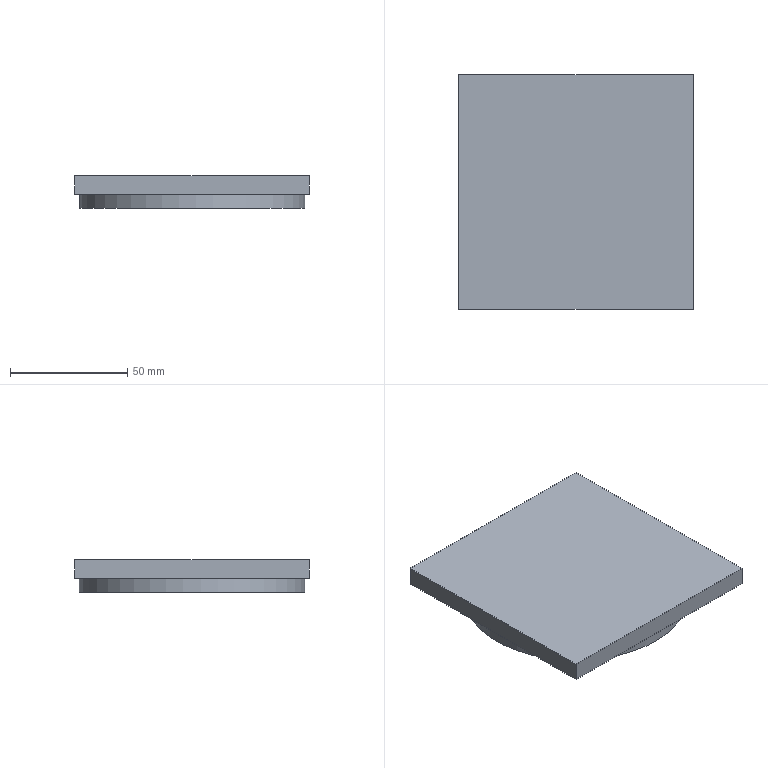Part | NX | 2 solids | 27 faces | box 100 x 100 x 14 mm | volume 81891 mm3 | cylinder 15 | plane 12 | commonest cylinder face diameters 4.3 x6 5.5 x3 11 x3 96 x2 48.3 x1
STEP:
#1=CARTESIAN_POINT('',(48.,0.,4.));
#2=VERTEX_POINT('',#1);
#3=CARTESIAN_POINT('',(0.,0.,4.));
#4=DIRECTION('',(0.,0.,1.));
#5=DIRECTION('',(1.,0.,0.));
#6=AXIS2_PLACEMENT_3D('',#3,#4,#5);
#7=CIRCLE('',#6,48.);
#8=EDGE_CURVE('',#2,#2,#7,.F.);
#9=ORIENTED_EDGE('',*,*,#8,.F.);
#10=EDGE_LOOP('',(#9));
#11=FACE_BOUND('',#10,.T.);
#12=CARTESIAN_POINT('',(48.,0.,0.));
#13=VERTEX_POINT('',#12);
#14=CARTESIAN_POINT('',(0.,0.,0.));
#15=DIRECTION('',(0.,0.,1.));
#16=DIRECTION('',(1.,0.,0.));
#17=AXIS2_PLACEMENT_3D('',#14,#15,#16);
#18=CIRCLE('',#17,48.);
#19=EDGE_CURVE('',#13,#13,#18,.T.);
#20=ORIENTED_EDGE('',*,*,#19,.F.);
#21=EDGE_LOOP('',(#20));
#22=FACE_BOUND('',#21,.T.);
#23=CARTESIAN_POINT('',(0.,0.,4.));
#24=DIRECTION('',(0.,0.,-1.));
#25=DIRECTION('',(-1.,0.,0.));
#26=AXIS2_PLACEMENT_3D('',#23,#24,#25);
#27=CYLINDRICAL_SURFACE('',#26,48.);
#28=ADVANCED_FACE('',(#11,#22),#27,.F.);
#29=ORIENTED_EDGE('',*,*,#8,.T.);
#30=EDGE_LOOP('',(#29));
#31=FACE_BOUND('',#30,.T.);
#32=CARTESIAN_POINT('',(0.,0.,4.));
#33=DIRECTION('',(0.,0.,1.));
#34=DIRECTION('',(1.,0.,0.));
#35=AXIS2_PLACEMENT_3D('',#32,#33,#34);
#36=PLANE('',#35);
#37=ADVANCED_FACE('',(#31),#36,.F.);
#38=CARTESIAN_POINT('',(50.,-50.,8.));
#39=VERTEX_POINT('',#38);
#40=CARTESIAN_POINT('',(50.,50.,8.));
#41=VERTEX_POINT('',#40);
#42=CARTESIAN_POINT('',(50.,-50.,8.));
#43=DIRECTION('',(0.,1.,0.));
#44=VECTOR('',#43,1000.);
#45=LINE('',#42,#44);
#46=EDGE_CURVE('',#39,#41,#45,.T.);
#47=ORIENTED_EDGE('',*,*,#46,.T.);
#48=CARTESIAN_POINT('',(-50.,50.,8.));
#49=VERTEX_POINT('',#48);
#50=CARTESIAN_POINT('',(50.,50.,8.));
#51=DIRECTION('',(-1.,0.,0.));
#52=VECTOR('',#51,1000.);
#53=LINE('',#50,#52);
#54=EDGE_CURVE('',#41,#49,#53,.T.);
#55=ORIENTED_EDGE('',*,*,#54,.T.);
#56=CARTESIAN_POINT('',(-50.,-50.,8.));
#57=VERTEX_POINT('',#56);
#58=CARTESIAN_POINT('',(-50.,50.,8.));
#59=DIRECTION('',(0.,-1.,0.));
#60=VECTOR('',#59,1000.);
#61=LINE('',#58,#60);
#62=EDGE_CURVE('',#49,#57,#61,.T.);
#63=ORIENTED_EDGE('',*,*,#62,.T.);
#64=CARTESIAN_POINT('',(-50.,-50.,8.));
#65=DIRECTION('',(1.,0.,0.));
#66=VECTOR('',#65,1000.);
#67=LINE('',#64,#66);
#68=EDGE_CURVE('',#57,#39,#67,.T.);
#69=ORIENTED_EDGE('',*,*,#68,.T.);
#70=EDGE_LOOP('',(#47,#55,#63,#69));
#71=FACE_BOUND('',#70,.T.);
#72=CARTESIAN_POINT('',(0.,0.,8.));
#73=DIRECTION('',(0.,0.,1.));
#74=DIRECTION('',(1.,0.,0.));
#75=AXIS2_PLACEMENT_3D('',#72,#73,#74);
#76=PLANE('',#75);
#77=ADVANCED_FACE('',(#71),#76,.T.);
#78=CARTESIAN_POINT('',(50.,50.,0.));
#79=VERTEX_POINT('',#78);
#80=CARTESIAN_POINT('',(-50.,50.,0.));
#81=VERTEX_POINT('',#80);
#82=CARTESIAN_POINT('',(50.,50.,0.));
#83=DIRECTION('',(-1.,0.,0.));
#84=VECTOR('',#83,1000.);
#85=LINE('',#82,#84);
#86=EDGE_CURVE('',#79,#81,#85,.T.);
#87=ORIENTED_EDGE('',*,*,#86,.T.);
#88=CARTESIAN_POINT('',(-50.,50.,8.));
#89=DIRECTION('',(0.,0.,-1.));
#90=VECTOR('',#89,1000.);
#91=LINE('',#88,#90);
#92=EDGE_CURVE('',#49,#81,#91,.T.);
#93=ORIENTED_EDGE('',*,*,#92,.F.);
#94=ORIENTED_EDGE('',*,*,#54,.F.);
#95=CARTESIAN_POINT('',(50.,50.,8.));
#96=DIRECTION('',(0.,0.,-1.));
#97=VECTOR('',#96,1000.);
#98=LINE('',#95,#97);
#99=EDGE_CURVE('',#41,#79,#98,.T.);
#100=ORIENTED_EDGE('',*,*,#99,.T.);
#101=EDGE_LOOP('',(#87,#93,#94,#100));
#102=FACE_BOUND('',#101,.T.);
#103=CARTESIAN_POINT('',(50.,50.,8.));
#104=DIRECTION('',(0.,-1.,0.));
#105=DIRECTION('',(0.,0.,-1.));
#106=AXIS2_PLACEMENT_3D('',#103,#104,#105);
#107=PLANE('',#106);
#108=ADVANCED_FACE('',(#102),#107,.F.);
#109=CARTESIAN_POINT('',(-50.,-50.,0.));
#110=VERTEX_POINT('',#109);
#111=CARTESIAN_POINT('',(-50.,50.,0.));
#112=DIRECTION('',(0.,-1.,0.));
#113=VECTOR('',#112,1000.);
#114=LINE('',#111,#113);
#115=EDGE_CURVE('',#81,#110,#114,.T.);
#116=ORIENTED_EDGE('',*,*,#115,.T.);
#117=CARTESIAN_POINT('',(-50.,-50.,8.));
#118=DIRECTION('',(0.,0.,-1.));
#119=VECTOR('',#118,1000.);
#120=LINE('',#117,#119);
#121=EDGE_CURVE('',#57,#110,#120,.T.);
#122=ORIENTED_EDGE('',*,*,#121,.F.);
#123=ORIENTED_EDGE('',*,*,#62,.F.);
#124=ORIENTED_EDGE('',*,*,#92,.T.);
#125=EDGE_LOOP('',(#116,#122,#123,#124));
#126=FACE_BOUND('',#125,.T.);
#127=CARTESIAN_POINT('',(-50.,50.,8.));
#128=DIRECTION('',(1.,0.,0.));
#129=DIRECTION('',(0.,0.,-1.));
#130=AXIS2_PLACEMENT_3D('',#127,#128,#129);
#131=PLANE('',#130);
#132=ADVANCED_FACE('',(#126),#131,.F.);
#133=CARTESIAN_POINT('',(50.,-50.,0.));
#134=VERTEX_POINT('',#133);
#135=CARTESIAN_POINT('',(-50.,-50.,0.));
#136=DIRECTION('',(1.,0.,0.));
#137=VECTOR('',#136,1000.);
#138=LINE('',#135,#137);
#139=EDGE_CURVE('',#110,#134,#138,.T.);
#140=ORIENTED_EDGE('',*,*,#139,.T.);
#141=CARTESIAN_POINT('',(50.,-50.,8.));
#142=DIRECTION('',(0.,0.,-1.));
#143=VECTOR('',#142,1000.);
#144=LINE('',#141,#143);
#145=EDGE_CURVE('',#39,#134,#144,.T.);
#146=ORIENTED_EDGE('',*,*,#145,.F.);
#147=ORIENTED_EDGE('',*,*,#68,.F.);
#148=ORIENTED_EDGE('',*,*,#121,.T.);
#149=EDGE_LOOP('',(#140,#146,#147,#148));
#150=FACE_BOUND('',#149,.T.);
#151=CARTESIAN_POINT('',(-50.,-50.,8.));
#152=DIRECTION('',(0.,1.,0.));
#153=DIRECTION('',(0.,0.,1.));
#154=AXIS2_PLACEMENT_3D('',#151,#152,#153);
#155=PLANE('',#154);
#156=ADVANCED_FACE('',(#150),#155,.F.);
#157=CARTESIAN_POINT('',(50.,-50.,0.));
#158=DIRECTION('',(0.,1.,0.));
#159=VECTOR('',#158,1000.);
#160=LINE('',#157,#159);
#161=EDGE_CURVE('',#134,#79,#160,.T.);
#162=ORIENTED_EDGE('',*,*,#161,.T.);
#163=ORIENTED_EDGE('',*,*,#99,.F.);
#164=ORIENTED_EDGE('',*,*,#46,.F.);
#165=ORIENTED_EDGE('',*,*,#145,.T.);
#166=EDGE_LOOP('',(#162,#163,#164,#165));
#167=FACE_BOUND('',#166,.T.);
#168=CARTESIAN_POINT('',(50.,-50.,8.));
#169=DIRECTION('',(-1.,0.,0.));
#170=DIRECTION('',(0.,0.,1.));
#171=AXIS2_PLACEMENT_3D('',#168,#169,#170);
#172=PLANE('',#171);
#173=ADVANCED_FACE('',(#167),#172,.F.);
#174=ORIENTED_EDGE('',*,*,#19,.T.);
#175=EDGE_LOOP('',(#174));
#176=FACE_BOUND('',#175,.T.);
#177=ORIENTED_EDGE('',*,*,#161,.F.);
#178=ORIENTED_EDGE('',*,*,#139,.F.);
#179=ORIENTED_EDGE('',*,*,#115,.F.);
#180=ORIENTED_EDGE('',*,*,#86,.F.);
#181=EDGE_LOOP('',(#177,#178,#179,#180));
#182=FACE_BOUND('',#181,.T.);
#183=CARTESIAN_POINT('',(0.,0.,0.));
#184=DIRECTION('',(0.,0.,1.));
#185=DIRECTION('',(1.,0.,0.));
#186=AXIS2_PLACEMENT_3D('',#183,#184,#185);
#187=PLANE('',#186);
#188=ADVANCED_FACE('',(#176,#182),#187,.F.);
#189=CLOSED_SHELL('',(#28,#37,#77,#108,#132,#156,#173,#188));
#190=MANIFOLD_SOLID_BREP('',#189);
#191=CARTESIAN_POINT('',(-22.225,-38.495,-6.));
#192=VERTEX_POINT('',#191);
#193=CARTESIAN_POINT('',(-20.85,-36.113,-6.));
#194=DIRECTION('',(0.,0.,1.));
#195=DIRECTION('',(-0.5,-0.866,0.));
#196=AXIS2_PLACEMENT_3D('',#193,#194,#195);
#197=CIRCLE('',#196,2.75);
#198=EDGE_CURVE('',#192,#192,#197,.T.);
#199=ORIENTED_EDGE('',*,*,#198,.F.);
#200=EDGE_LOOP('',(#199));
#201=FACE_BOUND('',#200,.T.);
#202=CARTESIAN_POINT('',(-18.1,-36.113,-3.));
#203=VERTEX_POINT('',#202);
#204=CARTESIAN_POINT('',(-20.85,-36.113,-3.));
#205=DIRECTION('',(0.,0.,1.));
#206=DIRECTION('',(1.,0.,0.));
#207=AXIS2_PLACEMENT_3D('',#204,#205,#206);
#208=CIRCLE('',#207,2.75);
#209=EDGE_CURVE('',#203,#203,#208,.F.);
#210=ORIENTED_EDGE('',*,*,#209,.F.);
#211=EDGE_LOOP('',(#210));
#212=FACE_BOUND('',#211,.T.);
#213=CARTESIAN_POINT('',(-20.85,-36.113,-6.));
#214=DIRECTION('',(0.,0.,1.));
#215=DIRECTION('',(1.,0.,0.));
#216=AXIS2_PLACEMENT_3D('',#213,#214,#215);
#217=CYLINDRICAL_SURFACE('',#216,2.75);
#218=ADVANCED_FACE('',(#201,#212),#217,.F.);
#219=CARTESIAN_POINT('',(44.45,0.,-6.));
#220=VERTEX_POINT('',#219);
#221=CARTESIAN_POINT('',(41.7,0.,-6.));
#222=DIRECTION('',(0.,0.,1.));
#223=DIRECTION('',(1.,0.,0.));
#224=AXIS2_PLACEMENT_3D('',#221,#222,#223);
#225=CIRCLE('',#224,2.75);
#226=EDGE_CURVE('',#220,#220,#225,.T.);
#227=ORIENTED_EDGE('',*,*,#226,.F.);
#228=EDGE_LOOP('',(#227));
#229=FACE_BOUND('',#228,.T.);
#230=CARTESIAN_POINT('',(44.45,0.,-3.));
#231=VERTEX_POINT('',#230);
#232=CARTESIAN_POINT('',(41.7,0.,-3.));
#233=DIRECTION('',(0.,0.,1.));
#234=DIRECTION('',(1.,0.,0.));
#235=AXIS2_PLACEMENT_3D('',#232,#233,#234);
#236=CIRCLE('',#235,2.75);
#237=EDGE_CURVE('',#231,#231,#236,.F.);
#238=ORIENTED_EDGE('',*,*,#237,.F.);
#239=EDGE_LOOP('',(#238));
#240=FACE_BOUND('',#239,.T.);
#241=CARTESIAN_POINT('',(41.7,0.,-6.));
#242=DIRECTION('',(0.,0.,1.));
#243=DIRECTION('',(1.,0.,0.));
#244=AXIS2_PLACEMENT_3D('',#241,#242,#243);
#245=CYLINDRICAL_SURFACE('',#244,2.75);
#246=ADVANCED_FACE('',(#229,#240),#245,.F.);
#247=CARTESIAN_POINT('',(-23.174,15.862,-6.));
#248=VERTEX_POINT('',#247);
#249=CARTESIAN_POINT('',(-24.249,14.,-6.));
#250=DIRECTION('',(0.,0.,1.));
#251=DIRECTION('',(0.5,0.866,0.));
#252=AXIS2_PLACEMENT_3D('',#249,#250,#251);
#253=CIRCLE('',#252,2.15);
#254=EDGE_CURVE('',#248,#248,#253,.T.);
#255=ORIENTED_EDGE('',*,*,#254,.F.);
#256=EDGE_LOOP('',(#255));
#257=FACE_BOUND('',#256,.T.);
#258=CARTESIAN_POINT('',(-23.174,15.862,0.));
#259=VERTEX_POINT('',#258);
#260=CARTESIAN_POINT('',(-24.249,14.,0.));
#261=DIRECTION('',(0.,0.,1.));
#262=DIRECTION('',(0.5,0.866,0.));
#263=AXIS2_PLACEMENT_3D('',#260,#261,#262);
#264=CIRCLE('',#263,2.15);
#265=EDGE_CURVE('',#259,#259,#264,.T.);
#266=ORIENTED_EDGE('',*,*,#265,.T.);
#267=EDGE_LOOP('',(#266));
#268=FACE_BOUND('',#267,.T.);
#269=CARTESIAN_POINT('',(-24.249,14.,-6.));
#270=DIRECTION('',(0.,0.,1.));
#271=DIRECTION('',(1.,0.,0.));
#272=AXIS2_PLACEMENT_3D('',#269,#270,#271);
#273=CYLINDRICAL_SURFACE('',#272,2.15);
#274=ADVANCED_FACE('',(#257,#268),#273,.F.);
#275=CARTESIAN_POINT('',(24.15,0.,-6.));
#276=VERTEX_POINT('',#275);
#277=CARTESIAN_POINT('',(0.,0.,-6.));
#278=DIRECTION('',(0.,0.,1.));
#279=DIRECTION('',(1.,0.,0.));
#280=AXIS2_PLACEMENT_3D('',#277,#278,#279);
#281=CIRCLE('',#280,24.15);
#282=EDGE_CURVE('',#276,#276,#281,.T.);
#283=ORIENTED_EDGE('',*,*,#282,.F.);
#284=EDGE_LOOP('',(#283));
#285=FACE_BOUND('',#284,.T.);
#286=CARTESIAN_POINT('',(24.15,0.,0.));
#287=VERTEX_POINT('',#286);
#288=CARTESIAN_POINT('',(0.,0.,0.));
#289=DIRECTION('',(0.,0.,1.));
#290=DIRECTION('',(1.,0.,0.));
#291=AXIS2_PLACEMENT_3D('',#288,#289,#290);
#292=CIRCLE('',#291,24.15);
#293=EDGE_CURVE('',#287,#287,#292,.T.);
#294=ORIENTED_EDGE('',*,*,#293,.T.);
#295=EDGE_LOOP('',(#294));
#296=FACE_BOUND('',#295,.T.);
#297=CARTESIAN_POINT('',(0.,0.,-6.));
#298=DIRECTION('',(0.,0.,1.));
#299=DIRECTION('',(1.,0.,0.));
#300=AXIS2_PLACEMENT_3D('',#297,#298,#299);
#301=CYLINDRICAL_SURFACE('',#300,24.15);
#302=ADVANCED_FACE('',(#285,#296),#301,.F.);
#303=CARTESIAN_POINT('',(-23.6,36.113,-3.));
#304=VERTEX_POINT('',#303);
#305=CARTESIAN_POINT('',(-20.85,36.113,-3.));
#306=DIRECTION('',(0.,0.,-1.));
#307=DIRECTION('',(-1.,0.,0.));
#308=AXIS2_PLACEMENT_3D('',#305,#306,#307);
#309=CIRCLE('',#308,2.75);
#310=EDGE_CURVE('',#304,#304,#309,.F.);
#311=ORIENTED_EDGE('',*,*,#310,.T.);
#312=EDGE_LOOP('',(#311));
#313=FACE_BOUND('',#312,.T.);
#314=CARTESIAN_POINT('',(-22.225,38.495,-6.));
#315=VERTEX_POINT('',#314);
#316=CARTESIAN_POINT('',(-20.85,36.113,-6.));
#317=DIRECTION('',(0.,0.,1.));
#318=DIRECTION('',(-0.5,0.866,0.));
#319=AXIS2_PLACEMENT_3D('',#316,#317,#318);
#320=CIRCLE('',#319,2.75);
#321=EDGE_CURVE('',#315,#315,#320,.T.);
#322=ORIENTED_EDGE('',*,*,#321,.F.);
#323=EDGE_LOOP('',(#322));
#324=FACE_BOUND('',#323,.T.);
#325=CARTESIAN_POINT('',(-20.85,36.113,-6.));
#326=DIRECTION('',(0.,0.,1.));
#327=DIRECTION('',(1.,0.,0.));
#328=AXIS2_PLACEMENT_3D('',#325,#326,#327);
#329=CYLINDRICAL_SURFACE('',#328,2.75);
#330=ADVANCED_FACE('',(#313,#324),#329,.F.);
#331=CARTESIAN_POINT('',(-2.15,-28.,-6.));
#332=VERTEX_POINT('',#331);
#333=CARTESIAN_POINT('',(0.,-28.,-6.));
#334=DIRECTION('',(0.,0.,1.));
#335=DIRECTION('',(-1.,0.,0.));
#336=AXIS2_PLACEMENT_3D('',#333,#334,#335);
#337=CIRCLE('',#336,2.15);
#338=EDGE_CURVE('',#332,#332,#337,.T.);
#339=ORIENTED_EDGE('',*,*,#338,.F.);
#340=EDGE_LOOP('',(#339));
#341=FACE_BOUND('',#340,.T.);
#342=CARTESIAN_POINT('',(-2.15,-28.,0.));
#343=VERTEX_POINT('',#342);
#344=CARTESIAN_POINT('',(0.,-28.,0.));
#345=DIRECTION('',(0.,0.,1.));
#346=DIRECTION('',(-1.,0.,0.));
#347=AXIS2_PLACEMENT_3D('',#344,#345,#346);
#348=CIRCLE('',#347,2.15);
#349=EDGE_CURVE('',#343,#343,#348,.T.);
#350=ORIENTED_EDGE('',*,*,#349,.T.);
#351=EDGE_LOOP('',(#350));
#352=FACE_BOUND('',#351,.T.);
#353=CARTESIAN_POINT('',(0.,-28.,-6.));
#354=DIRECTION('',(0.,0.,1.));
#355=DIRECTION('',(1.,0.,0.));
#356=AXIS2_PLACEMENT_3D('',#353,#354,#355);
#357=CYLINDRICAL_SURFACE('',#356,2.15);
#358=ADVANCED_FACE('',(#341,#352),#357,.F.);
#359=CARTESIAN_POINT('',(2.15,28.,-6.));
#360=VERTEX_POINT('',#359);
#361=CARTESIAN_POINT('',(0.,28.,-6.));
#362=DIRECTION('',(0.,0.,1.));
#363=DIRECTION('',(1.,0.,0.));
#364=AXIS2_PLACEMENT_3D('',#361,#362,#363);
#365=CIRCLE('',#364,2.15);
#366=EDGE_CURVE('',#360,#360,#365,.T.);
#367=ORIENTED_EDGE('',*,*,#366,.F.);
#368=EDGE_LOOP('',(#367));
#369=FACE_BOUND('',#368,.T.);
#370=CARTESIAN_POINT('',(2.15,28.,0.));
#371=VERTEX_POINT('',#370);
#372=CARTESIAN_POINT('',(0.,28.,0.));
#373=DIRECTION('',(0.,0.,1.));
#374=DIRECTION('',(1.,0.,0.));
#375=AXIS2_PLACEMENT_3D('',#372,#373,#374);
#376=CIRCLE('',#375,2.15);
#377=EDGE_CURVE('',#371,#371,#376,.T.);
#378=ORIENTED_EDGE('',*,*,#377,.T.);
#379=EDGE_LOOP('',(#378));
#380=FACE_BOUND('',#379,.T.);
#381=CARTESIAN_POINT('',(0.,28.,-6.));
#382=DIRECTION('',(0.,0.,1.));
#383=DIRECTION('',(1.,0.,0.));
#384=AXIS2_PLACEMENT_3D('',#381,#382,#383);
#385=CYLINDRICAL_SURFACE('',#384,2.15);
#386=ADVANCED_FACE('',(#369,#380),#385,.F.);
#387=CARTESIAN_POINT('',(23.174,-15.862,-6.));
#388=VERTEX_POINT('',#387);
#389=CARTESIAN_POINT('',(24.249,-14.,-6.));
#390=DIRECTION('',(0.,0.,1.));
#391=DIRECTION('',(-0.5,-0.866,0.));
#392=AXIS2_PLACEMENT_3D('',#389,#390,#391);
#393=CIRCLE('',#392,2.15);
#394=EDGE_CURVE('',#388,#388,#393,.T.);
#395=ORIENTED_EDGE('',*,*,#394,.F.);
#396=EDGE_LOOP('',(#395));
#397=FACE_BOUND('',#396,.T.);
#398=CARTESIAN_POINT('',(23.174,-15.862,0.));
#399=VERTEX_POINT('',#398);
#400=CARTESIAN_POINT('',(24.249,-14.,0.));
#401=DIRECTION('',(0.,0.,1.));
#402=DIRECTION('',(-0.5,-0.866,0.));
#403=AXIS2_PLACEMENT_3D('',#400,#401,#402);
#404=CIRCLE('',#403,2.15);
#405=EDGE_CURVE('',#399,#399,#404,.T.);
#406=ORIENTED_EDGE('',*,*,#405,.T.);
#407=EDGE_LOOP('',(#406));
#408=FACE_BOUND('',#407,.T.);
#409=CARTESIAN_POINT('',(24.249,-14.,-6.));
#410=DIRECTION('',(0.,0.,1.));
#411=DIRECTION('',(1.,0.,0.));
#412=AXIS2_PLACEMENT_3D('',#409,#410,#411);
#413=CYLINDRICAL_SURFACE('',#412,2.15);
#414=ADVANCED_FACE('',(#397,#408),#413,.F.);
#415=CARTESIAN_POINT('',(25.324,12.138,-6.));
#416=VERTEX_POINT('',#415);
#417=CARTESIAN_POINT('',(24.249,14.,-6.));
#418=DIRECTION('',(0.,0.,1.));
#419=DIRECTION('',(0.5,-0.866,0.));
#420=AXIS2_PLACEMENT_3D('',#417,#418,#419);
#421=CIRCLE('',#420,2.15);
#422=EDGE_CURVE('',#416,#416,#421,.T.);
#423=ORIENTED_EDGE('',*,*,#422,.F.);
#424=EDGE_LOOP('',(#423));
#425=FACE_BOUND('',#424,.T.);
#426=CARTESIAN_POINT('',(25.324,12.138,0.));
#427=VERTEX_POINT('',#426);
#428=CARTESIAN_POINT('',(24.249,14.,0.));
#429=DIRECTION('',(0.,0.,1.));
#430=DIRECTION('',(0.5,-0.866,0.));
#431=AXIS2_PLACEMENT_3D('',#428,#429,#430);
#432=CIRCLE('',#431,2.15);
#433=EDGE_CURVE('',#427,#427,#432,.T.);
#434=ORIENTED_EDGE('',*,*,#433,.T.);
#435=EDGE_LOOP('',(#434));
#436=FACE_BOUND('',#435,.T.);
#437=CARTESIAN_POINT('',(24.249,14.,-6.));
#438=DIRECTION('',(0.,0.,1.));
#439=DIRECTION('',(1.,0.,0.));
#440=AXIS2_PLACEMENT_3D('',#437,#438,#439);
#441=CYLINDRICAL_SURFACE('',#440,2.15);
#442=ADVANCED_FACE('',(#425,#436),#441,.F.);
#443=CARTESIAN_POINT('',(48.,0.,-6.));
#444=VERTEX_POINT('',#443);
#445=CARTESIAN_POINT('',(0.,0.,-6.));
#446=DIRECTION('',(0.,0.,1.));
#447=DIRECTION('',(1.,0.,0.));
#448=AXIS2_PLACEMENT_3D('',#445,#446,#447);
#449=CIRCLE('',#448,48.);
#450=EDGE_CURVE('',#444,#444,#449,.T.);
#451=ORIENTED_EDGE('',*,*,#450,.T.);
#452=EDGE_LOOP('',(#451));
#453=FACE_BOUND('',#452,.T.);
#454=CARTESIAN_POINT('',(48.,0.,0.));
#455=VERTEX_POINT('',#454);
#456=CARTESIAN_POINT('',(0.,0.,0.));
#457=DIRECTION('',(0.,0.,1.));
#458=DIRECTION('',(1.,0.,0.));
#459=AXIS2_PLACEMENT_3D('',#456,#457,#458);
#460=CIRCLE('',#459,48.);
#461=EDGE_CURVE('',#455,#455,#460,.T.);
#462=ORIENTED_EDGE('',*,*,#461,.F.);
#463=EDGE_LOOP('',(#462));
#464=FACE_BOUND('',#463,.T.);
#465=CARTESIAN_POINT('',(0.,0.,-6.));
#466=DIRECTION('',(0.,0.,1.));
#467=DIRECTION('',(1.,0.,0.));
#468=AXIS2_PLACEMENT_3D('',#465,#466,#467);
#469=CYLINDRICAL_SURFACE('',#468,48.);
#470=ADVANCED_FACE('',(#453,#464),#469,.T.);
#471=CARTESIAN_POINT('',(-25.324,-12.138,-6.));
#472=VERTEX_POINT('',#471);
#473=CARTESIAN_POINT('',(-24.249,-14.,-6.));
#474=DIRECTION('',(0.,0.,1.));
#475=DIRECTION('',(-0.5,0.866,0.));
#476=AXIS2_PLACEMENT_3D('',#473,#474,#475);
#477=CIRCLE('',#476,2.15);
#478=EDGE_CURVE('',#472,#472,#477,.T.);
#479=ORIENTED_EDGE('',*,*,#478,.F.);
#480=EDGE_LOOP('',(#479));
#481=FACE_BOUND('',#480,.T.);
#482=CARTESIAN_POINT('',(-25.324,-12.138,0.));
#483=VERTEX_POINT('',#482);
#484=CARTESIAN_POINT('',(-24.249,-14.,0.));
#485=DIRECTION('',(0.,0.,1.));
#486=DIRECTION('',(-0.5,0.866,0.));
#487=AXIS2_PLACEMENT_3D('',#484,#485,#486);
#488=CIRCLE('',#487,2.15);
#489=EDGE_CURVE('',#483,#483,#488,.T.);
#490=ORIENTED_EDGE('',*,*,#489,.T.);
#491=EDGE_LOOP('',(#490));
#492=FACE_BOUND('',#491,.T.);
#493=CARTESIAN_POINT('',(-24.249,-14.,-6.));
#494=DIRECTION('',(0.,0.,1.));
#495=DIRECTION('',(1.,0.,0.));
#496=AXIS2_PLACEMENT_3D('',#493,#494,#495);
#497=CYLINDRICAL_SURFACE('',#496,2.15);
#498=ADVANCED_FACE('',(#481,#492),#497,.F.);
#499=ORIENTED_EDGE('',*,*,#450,.F.);
#500=EDGE_LOOP('',(#499));
#501=FACE_BOUND('',#500,.T.);
#502=ORIENTED_EDGE('',*,*,#226,.T.);
#503=EDGE_LOOP('',(#502));
#504=FACE_BOUND('',#503,.T.);
#505=ORIENTED_EDGE('',*,*,#422,.T.);
#506=EDGE_LOOP('',(#505));
#507=FACE_BOUND('',#506,.T.);
#508=ORIENTED_EDGE('',*,*,#394,.T.);
#509=EDGE_LOOP('',(#508));
#510=FACE_BOUND('',#509,.T.);
#511=ORIENTED_EDGE('',*,*,#366,.T.);
#512=EDGE_LOOP('',(#511));
#513=FACE_BOUND('',#512,.T.);
#514=ORIENTED_EDGE('',*,*,#338,.T.);
#515=EDGE_LOOP('',(#514));
#516=FACE_BOUND('',#515,.T.);
#517=ORIENTED_EDGE('',*,*,#321,.T.);
#518=EDGE_LOOP('',(#517));
#519=FACE_BOUND('',#518,.T.);
#520=ORIENTED_EDGE('',*,*,#198,.T.);
#521=EDGE_LOOP('',(#520));
#522=FACE_BOUND('',#521,.T.);
#523=ORIENTED_EDGE('',*,*,#282,.T.);
#524=EDGE_LOOP('',(#523));
#525=FACE_BOUND('',#524,.T.);
#526=ORIENTED_EDGE('',*,*,#254,.T.);
#527=EDGE_LOOP('',(#526));
#528=FACE_BOUND('',#527,.T.);
#529=ORIENTED_EDGE('',*,*,#478,.T.);
#530=EDGE_LOOP('',(#529));
#531=FACE_BOUND('',#530,.T.);
#532=CARTESIAN_POINT('',(20.85,0.,-6.));
#533=DIRECTION('',(0.,0.,1.));
#534=DIRECTION('',(1.,0.,0.));
#535=AXIS2_PLACEMENT_3D('',#532,#533,#534);
#536=PLANE('',#535);
#537=ADVANCED_FACE('',(#501,#504,#507,#510,#513,#516,#519,#522,#525,#528,#531),#536,.F.);
#538=CARTESIAN_POINT('',(-23.6,40.876,-3.));
#539=VERTEX_POINT('',#538);
#540=CARTESIAN_POINT('',(-20.85,36.113,-3.));
#541=DIRECTION('',(0.,0.,-1.));
#542=DIRECTION('',(-0.5,0.866,0.));
#543=AXIS2_PLACEMENT_3D('',#540,#541,#542);
#544=CIRCLE('',#543,5.5);
#545=EDGE_CURVE('',#539,#539,#544,.F.);
#546=ORIENTED_EDGE('',*,*,#545,.T.);
#547=EDGE_LOOP('',(#546));
#548=FACE_BOUND('',#547,.T.);
#549=ORIENTED_EDGE('',*,*,#310,.F.);
#550=EDGE_LOOP('',(#549));
#551=FACE_BOUND('',#550,.T.);
#552=CARTESIAN_POINT('',(-20.85,36.113,-3.));
#553=DIRECTION('',(0.,0.,-1.));
#554=DIRECTION('',(-1.,0.,0.));
#555=AXIS2_PLACEMENT_3D('',#552,#553,#554);
#556=PLANE('',#555);
#557=ADVANCED_FACE('',(#548,#551),#556,.F.);
#558=ORIENTED_EDGE('',*,*,#545,.F.);
#559=EDGE_LOOP('',(#558));
#560=FACE_BOUND('',#559,.T.);
#561=CARTESIAN_POINT('',(-23.6,40.876,0.));
#562=VERTEX_POINT('',#561);
#563=CARTESIAN_POINT('',(-20.85,36.113,0.));
#564=DIRECTION('',(0.,0.,-1.));
#565=DIRECTION('',(-0.5,0.866,0.));
#566=AXIS2_PLACEMENT_3D('',#563,#564,#565);
#567=CIRCLE('',#566,5.5);
#568=EDGE_CURVE('',#562,#562,#567,.T.);
#569=ORIENTED_EDGE('',*,*,#568,.F.);
#570=EDGE_LOOP('',(#569));
#571=FACE_BOUND('',#570,.T.);
#572=CARTESIAN_POINT('',(-20.85,36.113,-3.));
#573=DIRECTION('',(0.,0.,1.));
#574=DIRECTION('',(1.,0.,0.));
#575=AXIS2_PLACEMENT_3D('',#572,#573,#574);
#576=CYLINDRICAL_SURFACE('',#575,5.5);
#577=ADVANCED_FACE('',(#560,#571),#576,.F.);
#578=CARTESIAN_POINT('',(-23.6,-40.876,-3.));
#579=VERTEX_POINT('',#578);
#580=CARTESIAN_POINT('',(-20.85,-36.113,-3.));
#581=DIRECTION('',(0.,0.,1.));
#582=DIRECTION('',(-0.5,-0.866,0.));
#583=AXIS2_PLACEMENT_3D('',#580,#581,#582);
#584=CIRCLE('',#583,5.5);
#585=EDGE_CURVE('',#579,#579,#584,.F.);
#586=ORIENTED_EDGE('',*,*,#585,.F.);
#587=EDGE_LOOP('',(#586));
#588=FACE_BOUND('',#587,.T.);
#589=ORIENTED_EDGE('',*,*,#209,.T.);
#590=EDGE_LOOP('',(#589));
#591=FACE_BOUND('',#590,.T.);
#592=CARTESIAN_POINT('',(-20.85,-36.113,-3.));
#593=DIRECTION('',(0.,0.,1.));
#594=DIRECTION('',(1.,0.,0.));
#595=AXIS2_PLACEMENT_3D('',#592,#593,#594);
#596=PLANE('',#595);
#597=ADVANCED_FACE('',(#588,#591),#596,.T.);
#598=ORIENTED_EDGE('',*,*,#585,.T.);
#599=EDGE_LOOP('',(#598));
#600=FACE_BOUND('',#599,.T.);
#601=CARTESIAN_POINT('',(-23.6,-40.876,0.));
#602=VERTEX_POINT('',#601);
#603=CARTESIAN_POINT('',(-20.85,-36.113,0.));
#604=DIRECTION('',(0.,0.,1.));
#605=DIRECTION('',(-0.5,-0.866,0.));
#606=AXIS2_PLACEMENT_3D('',#603,#604,#605);
#607=CIRCLE('',#606,5.5);
#608=EDGE_CURVE('',#602,#602,#607,.T.);
#609=ORIENTED_EDGE('',*,*,#608,.T.);
#610=EDGE_LOOP('',(#609));
#611=FACE_BOUND('',#610,.T.);
#612=CARTESIAN_POINT('',(-20.85,-36.113,-3.));
#613=DIRECTION('',(0.,0.,1.));
#614=DIRECTION('',(1.,0.,0.));
#615=AXIS2_PLACEMENT_3D('',#612,#613,#614);
#616=CYLINDRICAL_SURFACE('',#615,5.5);
#617=ADVANCED_FACE('',(#600,#611),#616,.F.);
#618=CARTESIAN_POINT('',(47.2,0.,-3.));
#619=VERTEX_POINT('',#618);
#620=CARTESIAN_POINT('',(41.7,0.,-3.));
#621=DIRECTION('',(0.,0.,1.));
#622=DIRECTION('',(1.,0.,0.));
#623=AXIS2_PLACEMENT_3D('',#620,#621,#622);
#624=CIRCLE('',#623,5.5);
#625=EDGE_CURVE('',#619,#619,#624,.F.);
#626=ORIENTED_EDGE('',*,*,#625,.F.);
#627=EDGE_LOOP('',(#626));
#628=FACE_BOUND('',#627,.T.);
#629=ORIENTED_EDGE('',*,*,#237,.T.);
#630=EDGE_LOOP('',(#629));
#631=FACE_BOUND('',#630,.T.);
#632=CARTESIAN_POINT('',(41.7,0.,-3.));
#633=DIRECTION('',(0.,0.,1.));
#634=DIRECTION('',(1.,0.,0.));
#635=AXIS2_PLACEMENT_3D('',#632,#633,#634);
#636=PLANE('',#635);
#637=ADVANCED_FACE('',(#628,#631),#636,.T.);
#638=ORIENTED_EDGE('',*,*,#625,.T.);
#639=EDGE_LOOP('',(#638));
#640=FACE_BOUND('',#639,.T.);
#641=CARTESIAN_POINT('',(47.2,0.,0.));
#642=VERTEX_POINT('',#641);
#643=CARTESIAN_POINT('',(41.7,0.,0.));
#644=DIRECTION('',(0.,0.,1.));
#645=DIRECTION('',(1.,0.,0.));
#646=AXIS2_PLACEMENT_3D('',#643,#644,#645);
#647=CIRCLE('',#646,5.5);
#648=EDGE_CURVE('',#642,#642,#647,.T.);
#649=ORIENTED_EDGE('',*,*,#648,.T.);
#650=EDGE_LOOP('',(#649));
#651=FACE_BOUND('',#650,.T.);
#652=CARTESIAN_POINT('',(41.7,0.,-3.));
#653=DIRECTION('',(0.,0.,1.));
#654=DIRECTION('',(1.,0.,0.));
#655=AXIS2_PLACEMENT_3D('',#652,#653,#654);
#656=CYLINDRICAL_SURFACE('',#655,5.5);
#657=ADVANCED_FACE('',(#640,#651),#656,.F.);
#658=ORIENTED_EDGE('',*,*,#648,.F.);
#659=EDGE_LOOP('',(#658));
#660=FACE_BOUND('',#659,.T.);
#661=ORIENTED_EDGE('',*,*,#489,.F.);
#662=EDGE_LOOP('',(#661));
#663=FACE_BOUND('',#662,.T.);
#664=ORIENTED_EDGE('',*,*,#265,.F.);
#665=EDGE_LOOP('',(#664));
#666=FACE_BOUND('',#665,.T.);
#667=ORIENTED_EDGE('',*,*,#293,.F.);
#668=EDGE_LOOP('',(#667));
#669=FACE_BOUND('',#668,.T.);
#670=ORIENTED_EDGE('',*,*,#349,.F.);
#671=EDGE_LOOP('',(#670));
#672=FACE_BOUND('',#671,.T.);
#673=ORIENTED_EDGE('',*,*,#377,.F.);
#674=EDGE_LOOP('',(#673));
#675=FACE_BOUND('',#674,.T.);
#676=ORIENTED_EDGE('',*,*,#405,.F.);
#677=EDGE_LOOP('',(#676));
#678=FACE_BOUND('',#677,.T.);
#679=ORIENTED_EDGE('',*,*,#433,.F.);
#680=EDGE_LOOP('',(#679));
#681=FACE_BOUND('',#680,.T.);
#682=ORIENTED_EDGE('',*,*,#608,.F.);
#683=EDGE_LOOP('',(#682));
#684=FACE_BOUND('',#683,.T.);
#685=ORIENTED_EDGE('',*,*,#461,.T.);
#686=EDGE_LOOP('',(#685));
#687=FACE_BOUND('',#686,.T.);
#688=ORIENTED_EDGE('',*,*,#568,.T.);
#689=EDGE_LOOP('',(#688));
#690=FACE_BOUND('',#689,.T.);
#691=CARTESIAN_POINT('',(0.,0.,0.));
#692=DIRECTION('',(0.,0.,1.));
#693=DIRECTION('',(1.,0.,0.));
#694=AXIS2_PLACEMENT_3D('',#691,#692,#693);
#695=PLANE('',#694);
#696=ADVANCED_FACE('',(#660,#663,#666,#669,#672,#675,#678,#681,#684,#687,#690),#695,.T.);
#697=CLOSED_SHELL('',(#218,#246,#274,#302,#330,#358,#386,#414,#442,#470,#498,#537,#557,#577,#597,#617,#637,#657,#696));
#698=MANIFOLD_SOLID_BREP('',#697);
#699=(LENGTH_UNIT()NAMED_UNIT(*)SI_UNIT(.MILLI.,.METRE.));
#700=UNCERTAINTY_MEASURE_WITH_UNIT(LENGTH_MEASURE(0.00001),#699,'','');
#701=(NAMED_UNIT(*)PLANE_ANGLE_UNIT()SI_UNIT($,.RADIAN.));
#702=(NAMED_UNIT(*)SI_UNIT($,.STERADIAN.)SOLID_ANGLE_UNIT());
#703=(GEOMETRIC_REPRESENTATION_CONTEXT(3)GLOBAL_UNCERTAINTY_ASSIGNED_CONTEXT((#700))GLOBAL_UNIT_ASSIGNED_CONTEXT((#699,#701,#702))REPRESENTATION_CONTEXT('',''));
#704=ADVANCED_BREP_SHAPE_REPRESENTATION('',(#190,#698),#703);